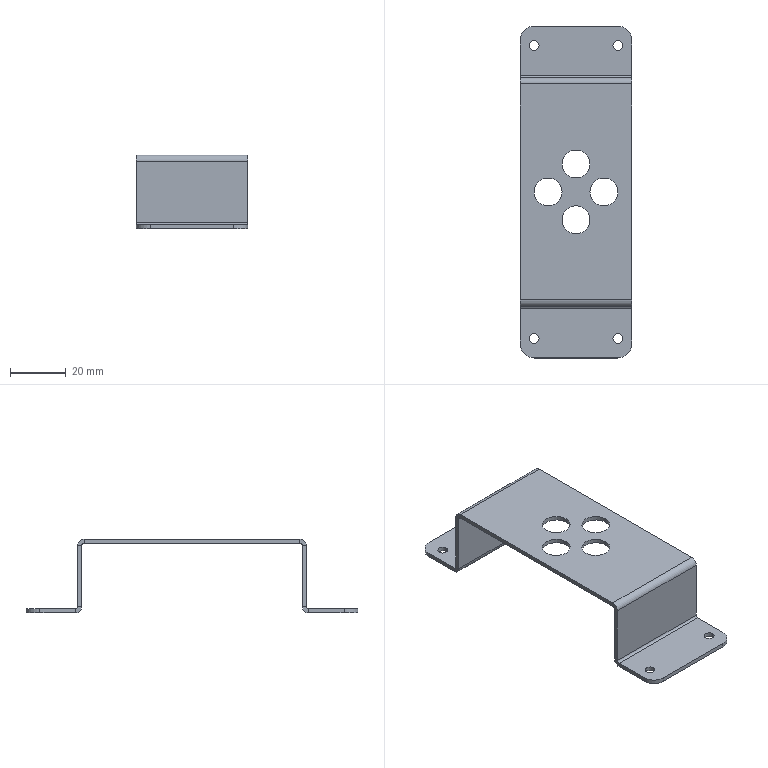Part | SolidWorks | features EdgeFlange 2, ICE 2, Fillet 1, FlatPattern 1, LPattern 1, RefAxis 1, SMBaseFlange 1, SheetMetal 1 | 1 solid | 58 faces | box 40 x 119 x 26.5 mm | volume 9419 mm3 | plane 30 | cylinder 28 | commonest cylinder face diameters 10 x12 3.5 x8 1.6 x4 4.6 x4